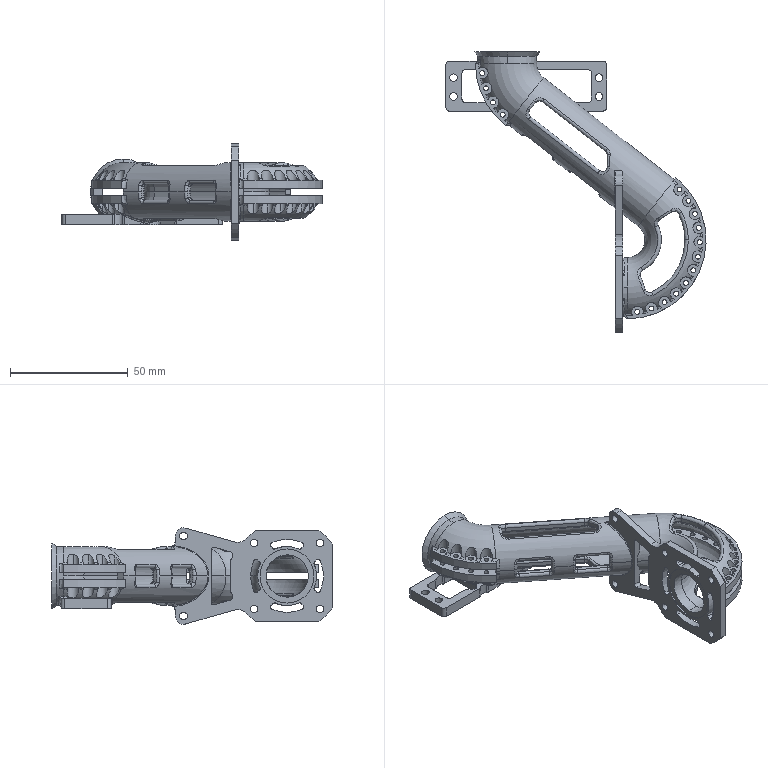Part | SolidWorks | features Fillet 19, ICE 17, Revolution 5, RevCut 2, Extrusion 1 | 1 solid | 570 faces | box 110.5 x 119.181 x 41 mm | volume 34590 mm3 | cylinder 292 | spline 95 | torus 91 | plane 90 | cone 2 | commonest cylinder face diameters 2.1 x64 5 x64 2 x55 3.2 x20 3 x19 4 x18